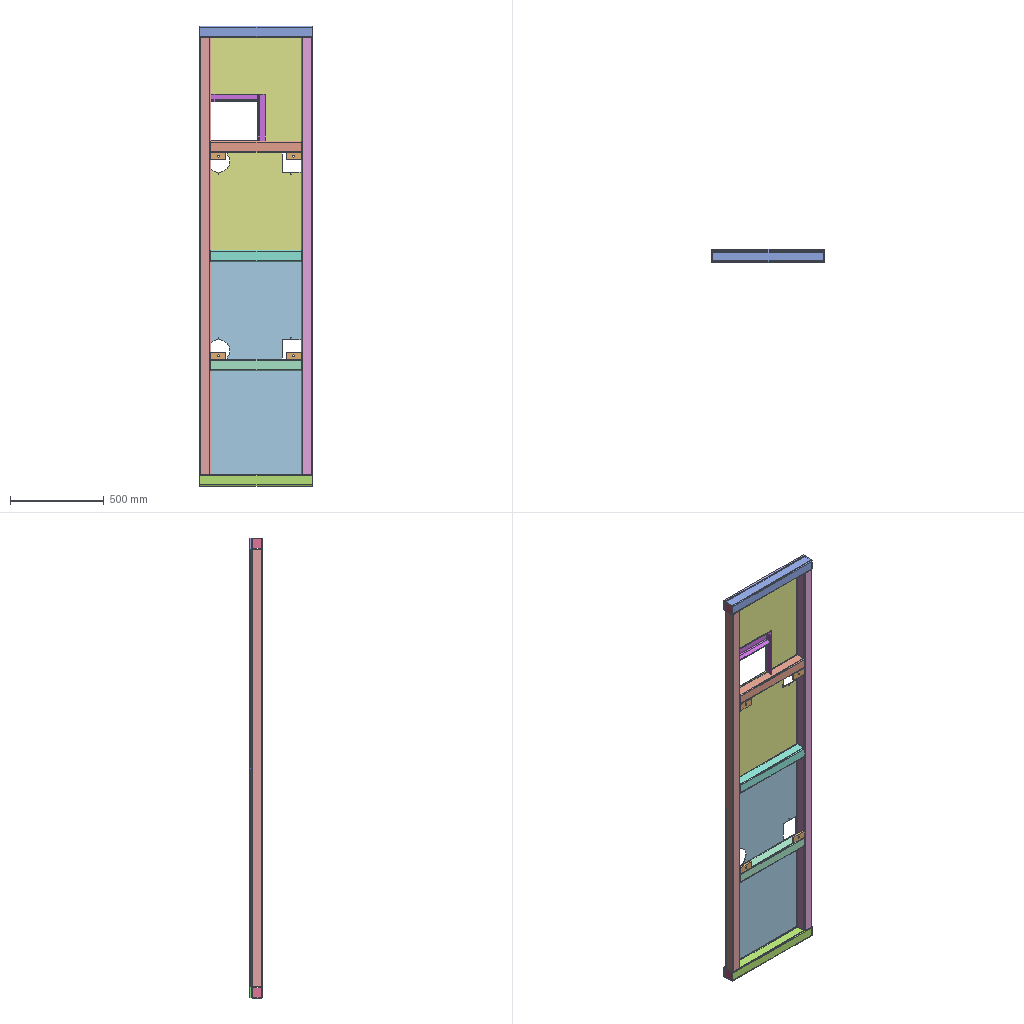Assembly | SolidWorks | 10 different items | 22 placed | box 600 x 70 x 2450 mm
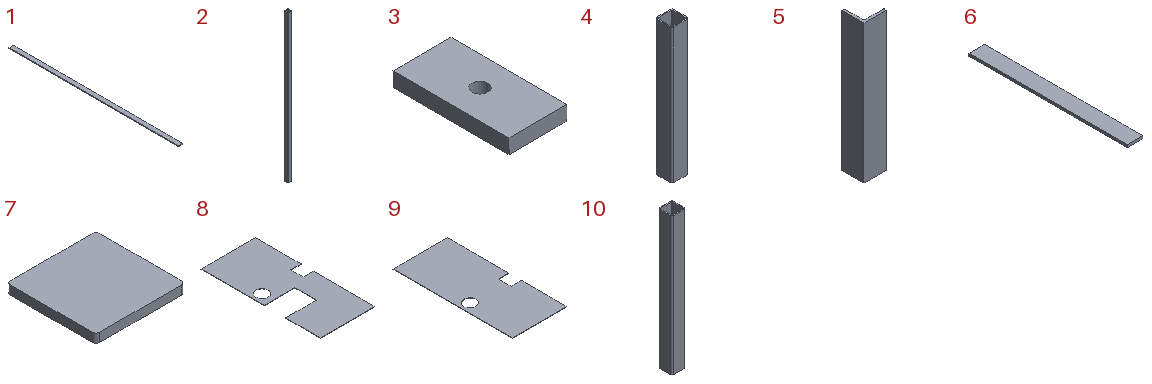Parts list (item | quantity | size | volume | features):
1 | x1 | 60 x 2330 x 10 mm | 1398000 mm3 | features Extrusion 1
2 | x2 | 60 x 60 x 2330 mm | 2033678 mm3 | features Fillet 2, Extrusion 1
3 | x4 | 40 x 80 x 10 mm | 31050 mm3 | features Extrusion 1, HoleWzd 1
4 | x3 | 60 x 60 x 480 mm | 418955 mm3 | features Fillet 2, Extrusion 1
5 | x2 | 40 x 40 x 250 mm | 77151 mm3 | features ICE 1, LibraryFeature 1
6 | x2 | 60 x 600 x 10 mm | 360000 mm3 | features Extrusion 1
7 | x4 | 50 x 50 x 5 mm | 12483 mm3 | features Fillet 2, ICE 2, Extrusion 1
8 | x1 | 530 x 1165 x 3 mm | 1593421 mm3 | features Extrusion 1, ICE 1
9 | x1 | 530 x 1165 x 3 mm | 1782421 mm3 | features Cut 1, Extrusion 1
10 | x2 | 60 x 60 x 600 mm | 523694 mm3 | features Fillet 2, Extrusion 1
Mates (type | each side: item.copy, entity, surface, feature):
Coincident | 2.1 face plane Boss-Extrude1 | 10.1 face plane | 3 times
Coincident | 2.1 face plane Boss-Extrude1 | 10.2 face plane | 3 times
Coincident | 10.1 face plane | 2.2 face plane | 3 times
Coincident | 2.1 face plane Boss-Extrude1 | 4.1 face plane Boss-Extrude1 | 2 times
Coincident | 2.1 face plane Boss-Extrude1 | 3.1 face plane Boss-Extrude1 | 2 times
Coincident | 2.1 face plane Boss-Extrude1 | 3.2 face plane Boss-Extrude1 | 2 times
Coincident | 2.2 face plane | 3.3 face plane Boss-Extrude1 | 2 times
Coincident | 3.2 face plane Boss-Extrude1 | 3.3 face plane Boss-Extrude1
Coincident | 2.2 face plane | 3.4 face plane Boss-Extrude1 | 2 times
Coincident | 3.1 face plane Boss-Extrude1 | 3.4 face plane Boss-Extrude1
Coincident | 10.1 face plane | 6.1 face plane | 3 times
Coincident | 10.2 face plane | 6.2 face plane | 3 times
DistanceDim | 7.1 face plane Boss-Extrude2 | 10.1 face plane | 2 times
Coincident | 10.1 face plane | 7.1 face plane Boss-Extrude2
DistanceDim | 7.2 face plane Boss-Extrude2 | 10.2 face plane | 2 times
Coincident | 10.2 face plane | 7.2 face plane Boss-Extrude2
Coincident | 2.1 face plane Boss-Extrude1 | 9.1 face plane
Coincident | 6.2 face plane | 9.1 face plane
Coincident | 6.1 face plane | 8.1 face plane
Width | 4.1 face plane Boss-Extrude1 | 4.1 face plane Boss-Extrude1 | 10.1 face plane | 10.2 face plane
Coincident | 4.2 face plane | 4.3 face plane | 2 times
DistanceDim | 4.2 face plane | 4.3 face plane
Coincident | 2.1 face plane Boss-Extrude1 | 4.3 face plane | 2 times
Width | 4.3 face plane | 4.2 face plane | 10.2 face plane | 10.1 face plane
Coincident | 3.3 face plane Boss-Extrude1 | 4.2 face plane
Coincident | 3.4 face plane Boss-Extrude1 | 4.3 face plane
Coincident | 5.1 face plane Boss-Extrude1 | 4.3 face plane | 2 times
DistanceDim | 5.1 face plane Boss-Extrude1 | 2.2 face plane
Coincident | 5.2 face plane Boss-Extrude1 | 5.1 face plane Boss-Extrude1 | 2 times
Coincident | 2.1 face plane Boss-Extrude1 | 5.2 face plane Boss-Extrude1
Coincident | 2.1 face plane Boss-Extrude1 | 8.1 face plane
Coincident | 2.2 face plane | 1.1 face plane | 2 times
Coincident | 6.1 face plane | 1.1 face plane
Coincident | 10.2 face plane | 7.3 face plane Boss-Extrude2
DistanceDim | 7.3 face plane Boss-Extrude2 | 10.2 face plane | 2 times
Coincident | 10.1 face plane | 7.4 face plane Boss-Extrude2
DistanceDim | 7.4 face plane Boss-Extrude2 | 10.1 face plane | 2 times